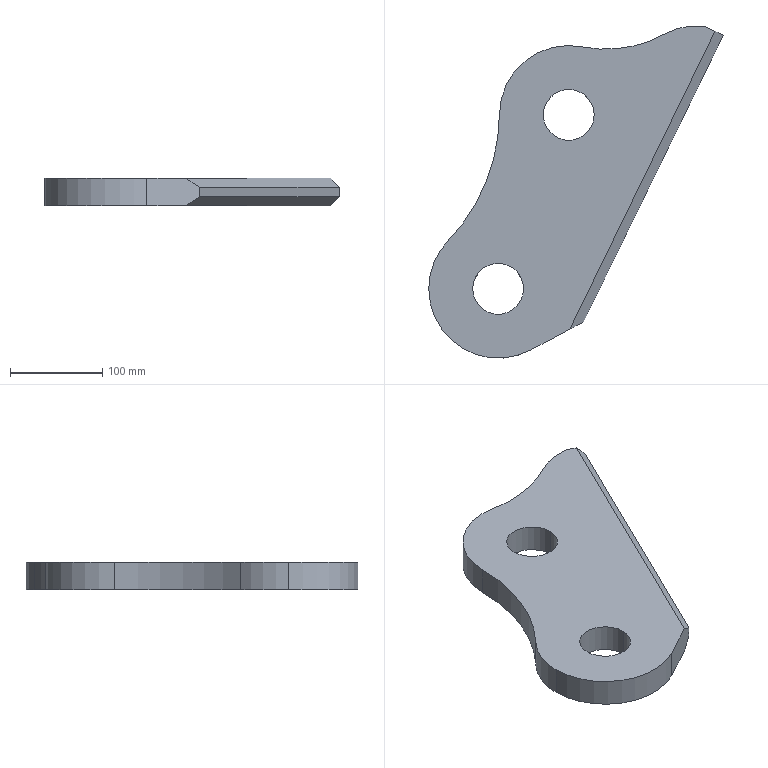Part | SolidWorks | features Chamfer 1, Extrusion 1 | 1 solid | 17 faces | box 318.374 x 359.351 x 30 mm | volume 1666573 mm3 | cylinder 10 | plane 7 | commonest cylinder face diameters 55 x4 150 x3 140 x1 260 x1 400 x1
STEP:
#1=CARTESIAN_POINT('',(-27.5,0.,30.));
#2=VERTEX_POINT('',#1);
#3=CARTESIAN_POINT('',(27.5,0.,30.));
#4=VERTEX_POINT('',#3);
#5=CARTESIAN_POINT('',(0.,0.,30.));
#6=DIRECTION('',(0.,0.,1.));
#7=DIRECTION('',(1.,0.,0.));
#8=AXIS2_PLACEMENT_3D('',#5,#6,#7);
#9=CIRCLE('',#8,27.5);
#10=EDGE_CURVE('',#2,#4,#9,.T.);
#11=ORIENTED_EDGE('',*,*,#10,.T.);
#12=CARTESIAN_POINT('',(27.5,0.,0.));
#13=VERTEX_POINT('',#12);
#14=CARTESIAN_POINT('',(27.5,0.,30.));
#15=DIRECTION('',(0.,0.,-1.));
#16=VECTOR('',#15,1000.);
#17=LINE('',#14,#16);
#18=EDGE_CURVE('',#4,#13,#17,.T.);
#19=ORIENTED_EDGE('',*,*,#18,.T.);
#20=CARTESIAN_POINT('',(-27.5,0.,0.));
#21=VERTEX_POINT('',#20);
#22=CARTESIAN_POINT('',(0.,0.,0.));
#23=DIRECTION('',(0.,0.,1.));
#24=DIRECTION('',(1.,0.,0.));
#25=AXIS2_PLACEMENT_3D('',#22,#23,#24);
#26=CIRCLE('',#25,27.5);
#27=EDGE_CURVE('',#21,#13,#26,.T.);
#28=ORIENTED_EDGE('',*,*,#27,.F.);
#29=CARTESIAN_POINT('',(-27.5,0.,30.));
#30=DIRECTION('',(0.,0.,-1.));
#31=VECTOR('',#30,1000.);
#32=LINE('',#29,#31);
#33=EDGE_CURVE('',#2,#21,#32,.T.);
#34=ORIENTED_EDGE('',*,*,#33,.F.);
#35=EDGE_LOOP('',(#11,#19,#28,#34));
#36=FACE_OUTER_BOUND('',#35,.T.);
#37=CARTESIAN_POINT('',(0.,0.,30.));
#38=DIRECTION('',(0.,0.,-1.));
#39=DIRECTION('',(-1.,0.,0.));
#40=AXIS2_PLACEMENT_3D('',#37,#38,#39);
#41=CYLINDRICAL_SURFACE('',#40,27.5);
#42=ADVANCED_FACE('',(#36),#41,.F.);
#43=CARTESIAN_POINT('',(48.874,188.085,30.));
#44=VERTEX_POINT('',#43);
#45=CARTESIAN_POINT('',(103.874,188.085,30.));
#46=VERTEX_POINT('',#45);
#47=CARTESIAN_POINT('',(76.374,188.085,30.));
#48=DIRECTION('',(0.,0.,1.));
#49=DIRECTION('',(1.,0.,0.));
#50=AXIS2_PLACEMENT_3D('',#47,#48,#49);
#51=CIRCLE('',#50,27.5);
#52=EDGE_CURVE('',#44,#46,#51,.T.);
#53=ORIENTED_EDGE('',*,*,#52,.T.);
#54=CARTESIAN_POINT('',(103.874,188.085,0.));
#55=VERTEX_POINT('',#54);
#56=CARTESIAN_POINT('',(103.874,188.085,30.));
#57=DIRECTION('',(0.,0.,-1.));
#58=VECTOR('',#57,1000.);
#59=LINE('',#56,#58);
#60=EDGE_CURVE('',#46,#55,#59,.T.);
#61=ORIENTED_EDGE('',*,*,#60,.T.);
#62=CARTESIAN_POINT('',(48.874,188.085,0.));
#63=VERTEX_POINT('',#62);
#64=CARTESIAN_POINT('',(76.374,188.085,0.));
#65=DIRECTION('',(0.,0.,1.));
#66=DIRECTION('',(1.,0.,0.));
#67=AXIS2_PLACEMENT_3D('',#64,#65,#66);
#68=CIRCLE('',#67,27.5);
#69=EDGE_CURVE('',#63,#55,#68,.T.);
#70=ORIENTED_EDGE('',*,*,#69,.F.);
#71=CARTESIAN_POINT('',(48.874,188.085,30.));
#72=DIRECTION('',(0.,0.,-1.));
#73=VECTOR('',#72,1000.);
#74=LINE('',#71,#73);
#75=EDGE_CURVE('',#44,#63,#74,.T.);
#76=ORIENTED_EDGE('',*,*,#75,.F.);
#77=EDGE_LOOP('',(#53,#61,#70,#76));
#78=FACE_OUTER_BOUND('',#77,.T.);
#79=CARTESIAN_POINT('',(76.374,188.085,30.));
#80=DIRECTION('',(0.,0.,-1.));
#81=DIRECTION('',(-1.,0.,0.));
#82=AXIS2_PLACEMENT_3D('',#79,#80,#81);
#83=CYLINDRICAL_SURFACE('',#82,27.5);
#84=ADVANCED_FACE('',(#78),#83,.F.);
#85=CARTESIAN_POINT('',(-75.,0.,30.));
#86=VERTEX_POINT('',#85);
#87=CARTESIAN_POINT('',(35.27,-66.189,30.));
#88=VERTEX_POINT('',#87);
#89=CARTESIAN_POINT('',(0.,0.,30.));
#90=DIRECTION('',(0.,0.,1.));
#91=DIRECTION('',(1.,0.,0.));
#92=AXIS2_PLACEMENT_3D('',#89,#90,#91);
#93=CIRCLE('',#92,75.);
#94=EDGE_CURVE('',#86,#88,#93,.T.);
#95=ORIENTED_EDGE('',*,*,#94,.F.);
#96=CARTESIAN_POINT('',(-75.,0.,0.));
#97=VERTEX_POINT('',#96);
#98=CARTESIAN_POINT('',(-75.,0.,30.));
#99=DIRECTION('',(0.,0.,-1.));
#100=VECTOR('',#99,1000.);
#101=LINE('',#98,#100);
#102=EDGE_CURVE('',#86,#97,#101,.T.);
#103=ORIENTED_EDGE('',*,*,#102,.T.);
#104=CARTESIAN_POINT('',(35.27,-66.189,0.));
#105=VERTEX_POINT('',#104);
#106=CARTESIAN_POINT('',(0.,0.,0.));
#107=DIRECTION('',(0.,0.,1.));
#108=DIRECTION('',(1.,0.,0.));
#109=AXIS2_PLACEMENT_3D('',#106,#107,#108);
#110=CIRCLE('',#109,75.);
#111=EDGE_CURVE('',#97,#105,#110,.T.);
#112=ORIENTED_EDGE('',*,*,#111,.T.);
#113=CARTESIAN_POINT('',(35.27,-66.189,30.));
#114=DIRECTION('',(0.,0.,-1.));
#115=VECTOR('',#114,1000.);
#116=LINE('',#113,#115);
#117=EDGE_CURVE('',#88,#105,#116,.T.);
#118=ORIENTED_EDGE('',*,*,#117,.F.);
#119=EDGE_LOOP('',(#95,#103,#112,#118));
#120=FACE_OUTER_BOUND('',#119,.T.);
#121=CARTESIAN_POINT('',(0.,0.,30.));
#122=DIRECTION('',(0.,0.,-1.));
#123=DIRECTION('',(-1.,0.,0.));
#124=AXIS2_PLACEMENT_3D('',#121,#122,#123);
#125=CYLINDRICAL_SURFACE('',#124,75.);
#126=ADVANCED_FACE('',(#120),#125,.T.);
#127=ORIENTED_EDGE('',*,*,#52,.F.);
#128=CARTESIAN_POINT('',(76.374,188.085,30.));
#129=DIRECTION('',(0.,0.,1.));
#130=DIRECTION('',(1.,0.,0.));
#131=AXIS2_PLACEMENT_3D('',#128,#129,#130);
#132=CIRCLE('',#131,27.5);
#133=EDGE_CURVE('',#46,#44,#132,.T.);
#134=ORIENTED_EDGE('',*,*,#133,.F.);
#135=EDGE_LOOP('',(#127,#134));
#136=FACE_BOUND('',#135,.T.);
#137=CARTESIAN_POINT('',(77.278,-43.804,30.));
#138=VERTEX_POINT('',#137);
#139=CARTESIAN_POINT('',(92.3,-35.8,30.));
#140=DIRECTION('',(0.8825,0.4703,0.));
#141=VECTOR('',#140,1000.);
#142=LINE('',#139,#141);
#143=EDGE_CURVE('',#88,#138,#142,.T.);
#144=ORIENTED_EDGE('',*,*,#143,.T.);
#145=CARTESIAN_POINT('',(234.383,278.764,30.));
#146=VERTEX_POINT('',#145);
#147=CARTESIAN_POINT('',(234.383,278.764,30.));
#148=DIRECTION('',(0.4379,0.899,0.));
#149=VECTOR('',#148,1000.);
#150=LINE('',#147,#149);
#151=EDGE_CURVE('',#138,#146,#150,.T.);
#152=ORIENTED_EDGE('',*,*,#151,.T.);
#153=CARTESIAN_POINT('',(224.494,283.581,30.));
#154=VERTEX_POINT('',#153);
#155=CARTESIAN_POINT('',(243.374,274.385,30.));
#156=DIRECTION('',(-0.899,0.4379,0.));
#157=VECTOR('',#156,1000.);
#158=LINE('',#155,#157);
#159=EDGE_CURVE('',#146,#154,#158,.T.);
#160=ORIENTED_EDGE('',*,*,#159,.T.);
#161=CARTESIAN_POINT('',(180.063,275.5,30.));
#162=VERTEX_POINT('',#161);
#163=CARTESIAN_POINT('',(214.134,214.351,30.));
#164=DIRECTION('',(0.,0.,1.));
#165=DIRECTION('',(1.,0.,0.));
#166=AXIS2_PLACEMENT_3D('',#163,#164,#165);
#167=CIRCLE('',#166,70.);
#168=EDGE_CURVE('',#154,#162,#167,.T.);
#169=ORIENTED_EDGE('',*,*,#168,.T.);
#170=CARTESIAN_POINT('',(91.16,261.613,30.));
#171=VERTEX_POINT('',#170);
#172=CARTESIAN_POINT('',(116.789,389.062,30.));
#173=DIRECTION('',(0.,0.,-1.));
#174=DIRECTION('',(1.,0.,0.));
#175=AXIS2_PLACEMENT_3D('',#172,#173,#174);
#176=CIRCLE('',#175,130.);
#177=EDGE_CURVE('',#162,#171,#176,.T.);
#178=ORIENTED_EDGE('',*,*,#177,.T.);
#179=CARTESIAN_POINT('',(1.376,188.662,30.));
#180=VERTEX_POINT('',#179);
#181=CARTESIAN_POINT('',(76.374,188.085,30.));
#182=DIRECTION('',(0.,0.,1.));
#183=DIRECTION('',(1.,0.,0.));
#184=AXIS2_PLACEMENT_3D('',#181,#182,#183);
#185=CIRCLE('',#184,75.);
#186=EDGE_CURVE('',#171,#180,#185,.T.);
#187=ORIENTED_EDGE('',*,*,#186,.T.);
#188=CARTESIAN_POINT('',(-54.169,51.873,30.));
#189=VERTEX_POINT('',#188);
#190=CARTESIAN_POINT('',(-198.618,190.199,30.));
#191=DIRECTION('',(0.,0.,-1.));
#192=DIRECTION('',(1.,0.,0.));
#193=AXIS2_PLACEMENT_3D('',#190,#191,#192);
#194=CIRCLE('',#193,200.);
#195=EDGE_CURVE('',#180,#189,#194,.T.);
#196=ORIENTED_EDGE('',*,*,#195,.T.);
#197=CARTESIAN_POINT('',(0.,0.,30.));
#198=DIRECTION('',(0.,0.,1.));
#199=DIRECTION('',(1.,0.,0.));
#200=AXIS2_PLACEMENT_3D('',#197,#198,#199);
#201=CIRCLE('',#200,75.);
#202=EDGE_CURVE('',#189,#86,#201,.T.);
#203=ORIENTED_EDGE('',*,*,#202,.T.);
#204=ORIENTED_EDGE('',*,*,#94,.T.);
#205=EDGE_LOOP('',(#144,#152,#160,#169,#178,#187,#196,#203,#204));
#206=FACE_OUTER_BOUND('',#205,.T.);
#207=ORIENTED_EDGE('',*,*,#10,.F.);
#208=CARTESIAN_POINT('',(0.,0.,30.));
#209=DIRECTION('',(0.,0.,1.));
#210=DIRECTION('',(1.,0.,0.));
#211=AXIS2_PLACEMENT_3D('',#208,#209,#210);
#212=CIRCLE('',#211,27.5);
#213=EDGE_CURVE('',#4,#2,#212,.T.);
#214=ORIENTED_EDGE('',*,*,#213,.F.);
#215=EDGE_LOOP('',(#207,#214));
#216=FACE_BOUND('',#215,.T.);
#217=CARTESIAN_POINT('',(0.,0.,30.));
#218=DIRECTION('',(0.,0.,1.));
#219=DIRECTION('',(1.,0.,0.));
#220=AXIS2_PLACEMENT_3D('',#217,#218,#219);
#221=PLANE('',#220);
#222=ADVANCED_FACE('',(#136,#206,#216),#221,.T.);
#223=ORIENTED_EDGE('',*,*,#69,.T.);
#224=CARTESIAN_POINT('',(76.374,188.085,0.));
#225=DIRECTION('',(0.,0.,1.));
#226=DIRECTION('',(1.,0.,0.));
#227=AXIS2_PLACEMENT_3D('',#224,#225,#226);
#228=CIRCLE('',#227,27.5);
#229=EDGE_CURVE('',#55,#63,#228,.T.);
#230=ORIENTED_EDGE('',*,*,#229,.T.);
#231=EDGE_LOOP('',(#223,#230));
#232=FACE_BOUND('',#231,.T.);
#233=CARTESIAN_POINT('',(234.383,278.764,0.));
#234=VERTEX_POINT('',#233);
#235=CARTESIAN_POINT('',(224.494,283.581,0.));
#236=VERTEX_POINT('',#235);
#237=CARTESIAN_POINT('',(243.374,274.385,0.));
#238=DIRECTION('',(-0.899,0.4379,0.));
#239=VECTOR('',#238,1000.);
#240=LINE('',#237,#239);
#241=EDGE_CURVE('',#234,#236,#240,.T.);
#242=ORIENTED_EDGE('',*,*,#241,.F.);
#243=CARTESIAN_POINT('',(77.278,-43.804,0.));
#244=VERTEX_POINT('',#243);
#245=CARTESIAN_POINT('',(79.706,-38.82,0.));
#246=DIRECTION('',(-0.4379,-0.899,0.));
#247=VECTOR('',#246,1000.);
#248=LINE('',#245,#247);
#249=EDGE_CURVE('',#234,#244,#248,.T.);
#250=ORIENTED_EDGE('',*,*,#249,.T.);
#251=CARTESIAN_POINT('',(92.3,-35.8,0.));
#252=DIRECTION('',(0.8825,0.4703,0.));
#253=VECTOR('',#252,1000.);
#254=LINE('',#251,#253);
#255=EDGE_CURVE('',#105,#244,#254,.T.);
#256=ORIENTED_EDGE('',*,*,#255,.F.);
#257=ORIENTED_EDGE('',*,*,#111,.F.);
#258=CARTESIAN_POINT('',(-54.169,51.873,0.));
#259=VERTEX_POINT('',#258);
#260=CARTESIAN_POINT('',(0.,0.,0.));
#261=DIRECTION('',(0.,0.,1.));
#262=DIRECTION('',(1.,0.,0.));
#263=AXIS2_PLACEMENT_3D('',#260,#261,#262);
#264=CIRCLE('',#263,75.);
#265=EDGE_CURVE('',#259,#97,#264,.T.);
#266=ORIENTED_EDGE('',*,*,#265,.F.);
#267=CARTESIAN_POINT('',(1.376,188.662,0.));
#268=VERTEX_POINT('',#267);
#269=CARTESIAN_POINT('',(-198.618,190.199,0.));
#270=DIRECTION('',(0.,0.,-1.));
#271=DIRECTION('',(1.,0.,0.));
#272=AXIS2_PLACEMENT_3D('',#269,#270,#271);
#273=CIRCLE('',#272,200.);
#274=EDGE_CURVE('',#268,#259,#273,.T.);
#275=ORIENTED_EDGE('',*,*,#274,.F.);
#276=CARTESIAN_POINT('',(91.16,261.613,0.));
#277=VERTEX_POINT('',#276);
#278=CARTESIAN_POINT('',(76.374,188.085,0.));
#279=DIRECTION('',(0.,0.,1.));
#280=DIRECTION('',(1.,0.,0.));
#281=AXIS2_PLACEMENT_3D('',#278,#279,#280);
#282=CIRCLE('',#281,75.);
#283=EDGE_CURVE('',#277,#268,#282,.T.);
#284=ORIENTED_EDGE('',*,*,#283,.F.);
#285=CARTESIAN_POINT('',(180.063,275.5,0.));
#286=VERTEX_POINT('',#285);
#287=CARTESIAN_POINT('',(116.789,389.062,0.));
#288=DIRECTION('',(0.,0.,-1.));
#289=DIRECTION('',(1.,0.,0.));
#290=AXIS2_PLACEMENT_3D('',#287,#288,#289);
#291=CIRCLE('',#290,130.);
#292=EDGE_CURVE('',#286,#277,#291,.T.);
#293=ORIENTED_EDGE('',*,*,#292,.F.);
#294=CARTESIAN_POINT('',(214.134,214.351,0.));
#295=DIRECTION('',(0.,0.,1.));
#296=DIRECTION('',(1.,0.,0.));
#297=AXIS2_PLACEMENT_3D('',#294,#295,#296);
#298=CIRCLE('',#297,70.);
#299=EDGE_CURVE('',#236,#286,#298,.T.);
#300=ORIENTED_EDGE('',*,*,#299,.F.);
#301=EDGE_LOOP('',(#242,#250,#256,#257,#266,#275,#284,#293,#300));
#302=FACE_OUTER_BOUND('',#301,.T.);
#303=ORIENTED_EDGE('',*,*,#27,.T.);
#304=CARTESIAN_POINT('',(0.,0.,0.));
#305=DIRECTION('',(0.,0.,1.));
#306=DIRECTION('',(1.,0.,0.));
#307=AXIS2_PLACEMENT_3D('',#304,#305,#306);
#308=CIRCLE('',#307,27.5);
#309=EDGE_CURVE('',#13,#21,#308,.T.);
#310=ORIENTED_EDGE('',*,*,#309,.T.);
#311=EDGE_LOOP('',(#303,#310));
#312=FACE_BOUND('',#311,.T.);
#313=CARTESIAN_POINT('',(0.,0.,0.));
#314=DIRECTION('',(0.,0.,1.));
#315=DIRECTION('',(1.,0.,0.));
#316=AXIS2_PLACEMENT_3D('',#313,#314,#315);
#317=PLANE('',#316);
#318=ADVANCED_FACE('',(#232,#302,#312),#317,.F.);
#319=ORIENTED_EDGE('',*,*,#255,.T.);
#320=CARTESIAN_POINT('',(92.3,-35.8,10.));
#321=VERTEX_POINT('',#320);
#322=CARTESIAN_POINT('',(92.3,-35.8,10.));
#323=DIRECTION('',(0.7609,0.4055,0.5066));
#324=VECTOR('',#323,1000.);
#325=LINE('',#322,#324);
#326=EDGE_CURVE('',#244,#321,#325,.T.);
#327=ORIENTED_EDGE('',*,*,#326,.T.);
#328=CARTESIAN_POINT('',(92.3,-35.8,20.));
#329=VERTEX_POINT('',#328);
#330=CARTESIAN_POINT('',(92.3,-35.8,30.));
#331=DIRECTION('',(0.,0.,-1.));
#332=VECTOR('',#331,1000.);
#333=LINE('',#330,#332);
#334=EDGE_CURVE('',#329,#321,#333,.T.);
#335=ORIENTED_EDGE('',*,*,#334,.F.);
#336=CARTESIAN_POINT('',(80.222,-42.236,28.041));
#337=DIRECTION('',(-0.7609,-0.4055,0.5066));
#338=VECTOR('',#337,1000.);
#339=LINE('',#336,#338);
#340=EDGE_CURVE('',#329,#138,#339,.T.);
#341=ORIENTED_EDGE('',*,*,#340,.T.);
#342=ORIENTED_EDGE('',*,*,#143,.F.);
#343=ORIENTED_EDGE('',*,*,#117,.T.);
#344=EDGE_LOOP('',(#319,#327,#335,#341,#342,#343));
#345=FACE_OUTER_BOUND('',#344,.T.);
#346=CARTESIAN_POINT('',(92.3,-35.8,30.));
#347=DIRECTION('',(-0.4703,0.8825,0.));
#348=DIRECTION('',(-0.8825,-0.4703,0.));
#349=AXIS2_PLACEMENT_3D('',#346,#347,#348);
#350=PLANE('',#349);
#351=ADVANCED_FACE('',(#345),#350,.F.);
#352=ORIENTED_EDGE('',*,*,#334,.T.);
#353=CARTESIAN_POINT('',(243.374,274.385,10.));
#354=VERTEX_POINT('',#353);
#355=CARTESIAN_POINT('',(92.3,-35.8,10.));
#356=DIRECTION('',(0.4379,0.899,0.));
#357=VECTOR('',#356,1000.);
#358=LINE('',#355,#357);
#359=EDGE_CURVE('',#321,#354,#358,.T.);
#360=ORIENTED_EDGE('',*,*,#359,.T.);
#361=CARTESIAN_POINT('',(243.374,274.385,20.));
#362=VERTEX_POINT('',#361);
#363=CARTESIAN_POINT('',(243.374,274.385,30.));
#364=DIRECTION('',(0.,0.,-1.));
#365=VECTOR('',#364,1000.);
#366=LINE('',#363,#365);
#367=EDGE_CURVE('',#362,#354,#366,.T.);
#368=ORIENTED_EDGE('',*,*,#367,.F.);
#369=CARTESIAN_POINT('',(92.3,-35.8,20.));
#370=DIRECTION('',(-0.4379,-0.899,0.));
#371=VECTOR('',#370,1000.);
#372=LINE('',#369,#371);
#373=EDGE_CURVE('',#362,#329,#372,.T.);
#374=ORIENTED_EDGE('',*,*,#373,.T.);
#375=EDGE_LOOP('',(#352,#360,#368,#374));
#376=FACE_OUTER_BOUND('',#375,.T.);
#377=CARTESIAN_POINT('',(92.3,-35.8,30.));
#378=DIRECTION('',(-0.899,0.4379,0.));
#379=DIRECTION('',(-0.4379,-0.899,0.));
#380=AXIS2_PLACEMENT_3D('',#377,#378,#379);
#381=PLANE('',#380);
#382=ADVANCED_FACE('',(#376),#381,.F.);
#383=ORIENTED_EDGE('',*,*,#367,.T.);
#384=CARTESIAN_POINT('',(243.374,274.385,10.));
#385=DIRECTION('',(-0.6357,0.3096,-0.7071));
#386=VECTOR('',#385,1000.);
#387=LINE('',#384,#386);
#388=EDGE_CURVE('',#354,#234,#387,.T.);
#389=ORIENTED_EDGE('',*,*,#388,.T.);
#390=ORIENTED_EDGE('',*,*,#241,.T.);
#391=CARTESIAN_POINT('',(224.494,283.581,30.));
#392=DIRECTION('',(0.,0.,-1.));
#393=VECTOR('',#392,1000.);
#394=LINE('',#391,#393);
#395=EDGE_CURVE('',#154,#236,#394,.T.);
#396=ORIENTED_EDGE('',*,*,#395,.F.);
#397=ORIENTED_EDGE('',*,*,#159,.F.);
#398=CARTESIAN_POINT('',(234.383,278.764,30.));
#399=DIRECTION('',(0.6357,-0.3096,-0.7071));
#400=VECTOR('',#399,1000.);
#401=LINE('',#398,#400);
#402=EDGE_CURVE('',#146,#362,#401,.T.);
#403=ORIENTED_EDGE('',*,*,#402,.T.);
#404=EDGE_LOOP('',(#383,#389,#390,#396,#397,#403));
#405=FACE_OUTER_BOUND('',#404,.T.);
#406=CARTESIAN_POINT('',(243.374,274.385,30.));
#407=DIRECTION('',(-0.4379,-0.899,0.));
#408=DIRECTION('',(0.899,-0.4379,0.));
#409=AXIS2_PLACEMENT_3D('',#406,#407,#408);
#410=PLANE('',#409);
#411=ADVANCED_FACE('',(#405),#410,.F.);
#412=ORIENTED_EDGE('',*,*,#299,.T.);
#413=CARTESIAN_POINT('',(180.063,275.5,30.));
#414=DIRECTION('',(0.,0.,-1.));
#415=VECTOR('',#414,1000.);
#416=LINE('',#413,#415);
#417=EDGE_CURVE('',#162,#286,#416,.T.);
#418=ORIENTED_EDGE('',*,*,#417,.F.);
#419=ORIENTED_EDGE('',*,*,#168,.F.);
#420=ORIENTED_EDGE('',*,*,#395,.T.);
#421=EDGE_LOOP('',(#412,#418,#419,#420));
#422=FACE_OUTER_BOUND('',#421,.T.);
#423=CARTESIAN_POINT('',(214.134,214.351,30.));
#424=DIRECTION('',(0.,0.,-1.));
#425=DIRECTION('',(-1.,0.,0.));
#426=AXIS2_PLACEMENT_3D('',#423,#424,#425);
#427=CYLINDRICAL_SURFACE('',#426,70.);
#428=ADVANCED_FACE('',(#422),#427,.T.);
#429=ORIENTED_EDGE('',*,*,#292,.T.);
#430=CARTESIAN_POINT('',(91.16,261.613,30.));
#431=DIRECTION('',(0.,0.,-1.));
#432=VECTOR('',#431,1000.);
#433=LINE('',#430,#432);
#434=EDGE_CURVE('',#171,#277,#433,.T.);
#435=ORIENTED_EDGE('',*,*,#434,.F.);
#436=ORIENTED_EDGE('',*,*,#177,.F.);
#437=ORIENTED_EDGE('',*,*,#417,.T.);
#438=EDGE_LOOP('',(#429,#435,#436,#437));
#439=FACE_OUTER_BOUND('',#438,.T.);
#440=CARTESIAN_POINT('',(116.789,389.062,30.));
#441=DIRECTION('',(0.,0.,-1.));
#442=DIRECTION('',(-1.,0.,0.));
#443=AXIS2_PLACEMENT_3D('',#440,#441,#442);
#444=CYLINDRICAL_SURFACE('',#443,130.);
#445=ADVANCED_FACE('',(#439),#444,.F.);
#446=ORIENTED_EDGE('',*,*,#283,.T.);
#447=CARTESIAN_POINT('',(1.376,188.662,30.));
#448=DIRECTION('',(0.,0.,-1.));
#449=VECTOR('',#448,1000.);
#450=LINE('',#447,#449);
#451=EDGE_CURVE('',#180,#268,#450,.T.);
#452=ORIENTED_EDGE('',*,*,#451,.F.);
#453=ORIENTED_EDGE('',*,*,#186,.F.);
#454=ORIENTED_EDGE('',*,*,#434,.T.);
#455=EDGE_LOOP('',(#446,#452,#453,#454));
#456=FACE_OUTER_BOUND('',#455,.T.);
#457=CARTESIAN_POINT('',(76.374,188.085,30.));
#458=DIRECTION('',(0.,0.,-1.));
#459=DIRECTION('',(-1.,0.,0.));
#460=AXIS2_PLACEMENT_3D('',#457,#458,#459);
#461=CYLINDRICAL_SURFACE('',#460,75.);
#462=ADVANCED_FACE('',(#456),#461,.T.);
#463=ORIENTED_EDGE('',*,*,#274,.T.);
#464=CARTESIAN_POINT('',(-54.169,51.873,30.));
#465=DIRECTION('',(0.,0.,-1.));
#466=VECTOR('',#465,1000.);
#467=LINE('',#464,#466);
#468=EDGE_CURVE('',#189,#259,#467,.T.);
#469=ORIENTED_EDGE('',*,*,#468,.F.);
#470=ORIENTED_EDGE('',*,*,#195,.F.);
#471=ORIENTED_EDGE('',*,*,#451,.T.);
#472=EDGE_LOOP('',(#463,#469,#470,#471));
#473=FACE_OUTER_BOUND('',#472,.T.);
#474=CARTESIAN_POINT('',(-198.618,190.199,30.));
#475=DIRECTION('',(0.,0.,-1.));
#476=DIRECTION('',(-1.,0.,0.));
#477=AXIS2_PLACEMENT_3D('',#474,#475,#476);
#478=CYLINDRICAL_SURFACE('',#477,200.);
#479=ADVANCED_FACE('',(#473),#478,.F.);
#480=ORIENTED_EDGE('',*,*,#102,.F.);
#481=ORIENTED_EDGE('',*,*,#202,.F.);
#482=ORIENTED_EDGE('',*,*,#468,.T.);
#483=ORIENTED_EDGE('',*,*,#265,.T.);
#484=EDGE_LOOP('',(#480,#481,#482,#483));
#485=FACE_OUTER_BOUND('',#484,.T.);
#486=CARTESIAN_POINT('',(0.,0.,30.));
#487=DIRECTION('',(0.,0.,-1.));
#488=DIRECTION('',(-1.,0.,0.));
#489=AXIS2_PLACEMENT_3D('',#486,#487,#488);
#490=CYLINDRICAL_SURFACE('',#489,75.);
#491=ADVANCED_FACE('',(#485),#490,.T.);
#492=ORIENTED_EDGE('',*,*,#60,.F.);
#493=ORIENTED_EDGE('',*,*,#133,.T.);
#494=ORIENTED_EDGE('',*,*,#75,.T.);
#495=ORIENTED_EDGE('',*,*,#229,.F.);
#496=EDGE_LOOP('',(#492,#493,#494,#495));
#497=FACE_OUTER_BOUND('',#496,.T.);
#498=CARTESIAN_POINT('',(76.374,188.085,30.));
#499=DIRECTION('',(0.,0.,-1.));
#500=DIRECTION('',(-1.,0.,0.));
#501=AXIS2_PLACEMENT_3D('',#498,#499,#500);
#502=CYLINDRICAL_SURFACE('',#501,27.5);
#503=ADVANCED_FACE('',(#497),#502,.F.);
#504=ORIENTED_EDGE('',*,*,#18,.F.);
#505=ORIENTED_EDGE('',*,*,#213,.T.);
#506=ORIENTED_EDGE('',*,*,#33,.T.);
#507=ORIENTED_EDGE('',*,*,#309,.F.);
#508=EDGE_LOOP('',(#504,#505,#506,#507));
#509=FACE_OUTER_BOUND('',#508,.T.);
#510=CARTESIAN_POINT('',(0.,0.,30.));
#511=DIRECTION('',(0.,0.,-1.));
#512=DIRECTION('',(-1.,0.,0.));
#513=AXIS2_PLACEMENT_3D('',#510,#511,#512);
#514=CYLINDRICAL_SURFACE('',#513,27.5);
#515=ADVANCED_FACE('',(#509),#514,.F.);
#516=ORIENTED_EDGE('',*,*,#326,.F.);
#517=ORIENTED_EDGE('',*,*,#249,.F.);
#518=ORIENTED_EDGE('',*,*,#388,.F.);
#519=ORIENTED_EDGE('',*,*,#359,.F.);
#520=EDGE_LOOP('',(#516,#517,#518,#519));
#521=FACE_OUTER_BOUND('',#520,.T.);
#522=CARTESIAN_POINT('',(92.3,-35.8,10.));
#523=DIRECTION('',(-0.6357,0.3096,0.7071));
#524=DIRECTION('',(0.7436,0.,0.6686));
#525=AXIS2_PLACEMENT_3D('',#522,#523,#524);
#526=PLANE('',#525);
#527=ADVANCED_FACE('',(#521),#526,.F.);
#528=ORIENTED_EDGE('',*,*,#340,.F.);
#529=ORIENTED_EDGE('',*,*,#373,.F.);
#530=ORIENTED_EDGE('',*,*,#402,.F.);
#531=ORIENTED_EDGE('',*,*,#151,.F.);
#532=EDGE_LOOP('',(#528,#529,#530,#531));
#533=FACE_OUTER_BOUND('',#532,.T.);
#534=CARTESIAN_POINT('',(79.706,-38.82,30.));
#535=DIRECTION('',(0.6357,-0.3096,0.7071));
#536=DIRECTION('',(0.7436,0.,-0.6686));
#537=AXIS2_PLACEMENT_3D('',#534,#535,#536);
#538=PLANE('',#537);
#539=ADVANCED_FACE('',(#533),#538,.T.);
#540=CLOSED_SHELL('',(#42,#84,#126,#222,#318,#351,#382,#411,#428,#445,#462,#479,#491,#503,#515,#527,#539));
#541=MANIFOLD_SOLID_BREP('',#540);
#542=CARTESIAN_POINT('',(0.,0.,0.));
#543=DIRECTION('',(0.,0.,1.));
#544=DIRECTION('',(1.,0.,0.));
#545=AXIS2_PLACEMENT_3D('',#542,#543,#544);
#546=(LENGTH_UNIT()NAMED_UNIT(*)SI_UNIT(.MILLI.,.METRE.));
#547=UNCERTAINTY_MEASURE_WITH_UNIT(LENGTH_MEASURE(0.00001),#546,'','');
#548=(NAMED_UNIT(*)PLANE_ANGLE_UNIT()SI_UNIT($,.RADIAN.));
#549=(NAMED_UNIT(*)SI_UNIT($,.STERADIAN.)SOLID_ANGLE_UNIT());
#550=(GEOMETRIC_REPRESENTATION_CONTEXT(3)GLOBAL_UNCERTAINTY_ASSIGNED_CONTEXT((#547))GLOBAL_UNIT_ASSIGNED_CONTEXT((#546,#548,#549))REPRESENTATION_CONTEXT('',''));
#551=ADVANCED_BREP_SHAPE_REPRESENTATION('',(#541,#545),#550);